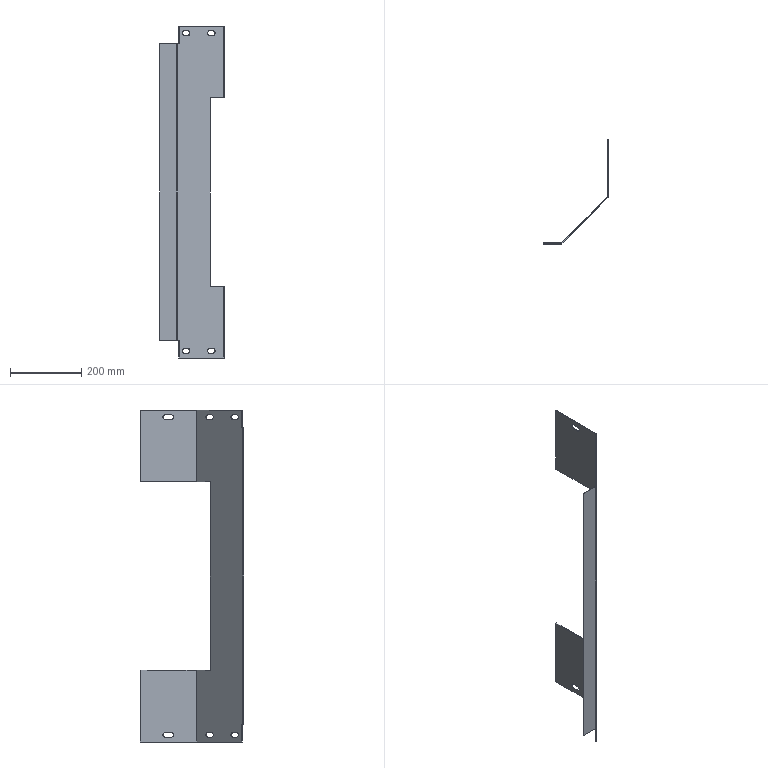Part | SolidWorks | features BaseBody 1 | 1 solid | 60 faces | box 181.421 x 291.421 x 932 mm | volume 492157 mm3 | plane 36 | cylinder 24 | commonest cylinder face diameters 13 x18 4 x3 8 x3